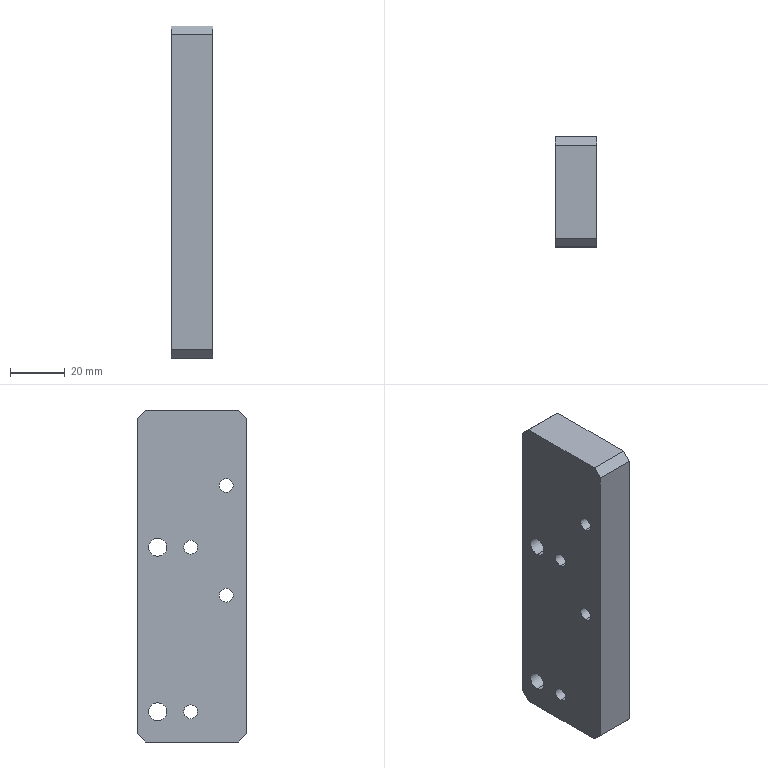Part | SolidWorks | features HoleWzd 4, Chamfer 1, Extrusion 1 | 1 solid | 44 faces | box 15 x 40 x 121 mm | volume 68938 mm3 | cylinder 20 | cone 12 | plane 12 | commonest cylinder face diameters 5 x8 4.2 x4 6.6 x4 11 x4
STEP:
#1=CARTESIAN_POINT('',(14.8,0.5,13.));
#2=VERTEX_POINT('',#1);
#3=CARTESIAN_POINT('',(14.8,0.5,8.));
#4=VERTEX_POINT('',#3);
#5=CARTESIAN_POINT('',(14.8,0.5,10.5));
#6=DIRECTION('',(1.,0.,0.));
#7=DIRECTION('',(0.,0.,-1.));
#8=AXIS2_PLACEMENT_3D('',#5,#6,#7);
#9=CIRCLE('',#8,2.5);
#10=EDGE_CURVE('',#2,#4,#9,.T.);
#11=ORIENTED_EDGE('',*,*,#10,.F.);
#12=CARTESIAN_POINT('',(15.,0.5,13.2));
#13=VERTEX_POINT('',#12);
#14=CARTESIAN_POINT('',(15.,0.5,13.2));
#15=DIRECTION('',(0.7071,0.,0.7071));
#16=VECTOR('',#15,1000.);
#17=LINE('',#14,#16);
#18=EDGE_CURVE('',#2,#13,#17,.T.);
#19=ORIENTED_EDGE('',*,*,#18,.T.);
#20=CARTESIAN_POINT('',(15.,0.5,7.8));
#21=VERTEX_POINT('',#20);
#22=CARTESIAN_POINT('',(15.,0.5,10.5));
#23=DIRECTION('',(1.,0.,0.));
#24=DIRECTION('',(0.,0.,-1.));
#25=AXIS2_PLACEMENT_3D('',#22,#23,#24);
#26=CIRCLE('',#25,2.7);
#27=EDGE_CURVE('',#13,#21,#26,.T.);
#28=ORIENTED_EDGE('',*,*,#27,.T.);
#29=CARTESIAN_POINT('',(15.,0.5,7.8));
#30=DIRECTION('',(0.7071,0.,-0.7071));
#31=VECTOR('',#30,1000.);
#32=LINE('',#29,#31);
#33=EDGE_CURVE('',#4,#21,#32,.T.);
#34=ORIENTED_EDGE('',*,*,#33,.F.);
#35=EDGE_LOOP('',(#11,#19,#28,#34));
#36=FACE_OUTER_BOUND('',#35,.T.);
#37=CARTESIAN_POINT('',(15.,0.5,10.5));
#38=DIRECTION('',(1.,0.,0.));
#39=DIRECTION('',(0.,0.,-1.));
#40=AXIS2_PLACEMENT_3D('',#37,#38,#39);
#41=CONICAL_SURFACE('',#40,2.7,0.7854);
#42=ADVANCED_FACE('',(#36),#41,.F.);
#43=CARTESIAN_POINT('',(0.,0.5,13.));
#44=VERTEX_POINT('',#43);
#45=CARTESIAN_POINT('',(0.,0.5,8.));
#46=VERTEX_POINT('',#45);
#47=CARTESIAN_POINT('',(0.,0.5,10.5));
#48=DIRECTION('',(1.,0.,0.));
#49=DIRECTION('',(0.,0.,-1.));
#50=AXIS2_PLACEMENT_3D('',#47,#48,#49);
#51=CIRCLE('',#50,2.5);
#52=EDGE_CURVE('',#44,#46,#51,.T.);
#53=ORIENTED_EDGE('',*,*,#52,.F.);
#54=CARTESIAN_POINT('',(15.,0.5,13.));
#55=DIRECTION('',(1.,0.,0.));
#56=VECTOR('',#55,1000.);
#57=LINE('',#54,#56);
#58=EDGE_CURVE('',#44,#2,#57,.T.);
#59=ORIENTED_EDGE('',*,*,#58,.T.);
#60=ORIENTED_EDGE('',*,*,#10,.T.);
#61=CARTESIAN_POINT('',(15.,0.5,8.));
#62=DIRECTION('',(1.,0.,0.));
#63=VECTOR('',#62,1000.);
#64=LINE('',#61,#63);
#65=EDGE_CURVE('',#46,#4,#64,.T.);
#66=ORIENTED_EDGE('',*,*,#65,.F.);
#67=EDGE_LOOP('',(#53,#59,#60,#66));
#68=FACE_OUTER_BOUND('',#67,.T.);
#69=CARTESIAN_POINT('',(15.,0.5,10.5));
#70=DIRECTION('',(1.,0.,0.));
#71=DIRECTION('',(0.,0.,-1.));
#72=AXIS2_PLACEMENT_3D('',#69,#70,#71);
#73=CYLINDRICAL_SURFACE('',#72,2.5);
#74=ADVANCED_FACE('',(#68),#73,.F.);
#75=CARTESIAN_POINT('',(14.8,0.5,-47.));
#76=VERTEX_POINT('',#75);
#77=CARTESIAN_POINT('',(14.8,0.5,-52.));
#78=VERTEX_POINT('',#77);
#79=CARTESIAN_POINT('',(14.8,0.5,-49.5));
#80=DIRECTION('',(1.,0.,0.));
#81=DIRECTION('',(0.,0.,-1.));
#82=AXIS2_PLACEMENT_3D('',#79,#80,#81);
#83=CIRCLE('',#82,2.5);
#84=EDGE_CURVE('',#76,#78,#83,.T.);
#85=ORIENTED_EDGE('',*,*,#84,.F.);
#86=CARTESIAN_POINT('',(15.,0.5,-46.8));
#87=VERTEX_POINT('',#86);
#88=CARTESIAN_POINT('',(15.,0.5,-46.8));
#89=DIRECTION('',(0.7071,0.,0.7071));
#90=VECTOR('',#89,1000.);
#91=LINE('',#88,#90);
#92=EDGE_CURVE('',#76,#87,#91,.T.);
#93=ORIENTED_EDGE('',*,*,#92,.T.);
#94=CARTESIAN_POINT('',(15.,0.5,-52.2));
#95=VERTEX_POINT('',#94);
#96=CARTESIAN_POINT('',(15.,0.5,-49.5));
#97=DIRECTION('',(1.,0.,0.));
#98=DIRECTION('',(0.,0.,-1.));
#99=AXIS2_PLACEMENT_3D('',#96,#97,#98);
#100=CIRCLE('',#99,2.7);
#101=EDGE_CURVE('',#87,#95,#100,.T.);
#102=ORIENTED_EDGE('',*,*,#101,.T.);
#103=CARTESIAN_POINT('',(15.,0.5,-52.2));
#104=DIRECTION('',(0.7071,0.,-0.7071));
#105=VECTOR('',#104,1000.);
#106=LINE('',#103,#105);
#107=EDGE_CURVE('',#78,#95,#106,.T.);
#108=ORIENTED_EDGE('',*,*,#107,.F.);
#109=EDGE_LOOP('',(#85,#93,#102,#108));
#110=FACE_OUTER_BOUND('',#109,.T.);
#111=CARTESIAN_POINT('',(15.,0.5,-49.5));
#112=DIRECTION('',(1.,0.,0.));
#113=DIRECTION('',(0.,0.,-1.));
#114=AXIS2_PLACEMENT_3D('',#111,#112,#113);
#115=CONICAL_SURFACE('',#114,2.7,0.7854);
#116=ADVANCED_FACE('',(#110),#115,.F.);
#117=CARTESIAN_POINT('',(0.,0.5,-47.));
#118=VERTEX_POINT('',#117);
#119=CARTESIAN_POINT('',(0.,0.5,-52.));
#120=VERTEX_POINT('',#119);
#121=CARTESIAN_POINT('',(0.,0.5,-49.5));
#122=DIRECTION('',(1.,0.,0.));
#123=DIRECTION('',(0.,0.,-1.));
#124=AXIS2_PLACEMENT_3D('',#121,#122,#123);
#125=CIRCLE('',#124,2.5);
#126=EDGE_CURVE('',#118,#120,#125,.T.);
#127=ORIENTED_EDGE('',*,*,#126,.F.);
#128=CARTESIAN_POINT('',(15.,0.5,-47.));
#129=DIRECTION('',(1.,0.,0.));
#130=VECTOR('',#129,1000.);
#131=LINE('',#128,#130);
#132=EDGE_CURVE('',#118,#76,#131,.T.);
#133=ORIENTED_EDGE('',*,*,#132,.T.);
#134=ORIENTED_EDGE('',*,*,#84,.T.);
#135=CARTESIAN_POINT('',(15.,0.5,-52.));
#136=DIRECTION('',(1.,0.,0.));
#137=VECTOR('',#136,1000.);
#138=LINE('',#135,#137);
#139=EDGE_CURVE('',#120,#78,#138,.T.);
#140=ORIENTED_EDGE('',*,*,#139,.F.);
#141=EDGE_LOOP('',(#127,#133,#134,#140));
#142=FACE_OUTER_BOUND('',#141,.T.);
#143=CARTESIAN_POINT('',(15.,0.5,-49.5));
#144=DIRECTION('',(1.,0.,0.));
#145=DIRECTION('',(0.,0.,-1.));
#146=AXIS2_PLACEMENT_3D('',#143,#144,#145);
#147=CYLINDRICAL_SURFACE('',#146,2.5);
#148=ADVANCED_FACE('',(#142),#147,.F.);
#149=CARTESIAN_POINT('',(8.2,12.5,16.));
#150=VERTEX_POINT('',#149);
#151=CARTESIAN_POINT('',(8.2,12.5,5.));
#152=VERTEX_POINT('',#151);
#153=CARTESIAN_POINT('',(8.2,12.5,10.5));
#154=DIRECTION('',(1.,0.,0.));
#155=DIRECTION('',(0.,0.,-1.));
#156=AXIS2_PLACEMENT_3D('',#153,#154,#155);
#157=CIRCLE('',#156,5.5);
#158=EDGE_CURVE('',#150,#152,#157,.T.);
#159=ORIENTED_EDGE('',*,*,#158,.F.);
#160=CARTESIAN_POINT('',(15.,12.5,16.));
#161=VERTEX_POINT('',#160);
#162=CARTESIAN_POINT('',(15.,12.5,16.));
#163=DIRECTION('',(1.,0.,0.));
#164=VECTOR('',#163,1000.);
#165=LINE('',#162,#164);
#166=EDGE_CURVE('',#150,#161,#165,.T.);
#167=ORIENTED_EDGE('',*,*,#166,.T.);
#168=CARTESIAN_POINT('',(15.,12.5,5.));
#169=VERTEX_POINT('',#168);
#170=CARTESIAN_POINT('',(15.,12.5,10.5));
#171=DIRECTION('',(1.,0.,0.));
#172=DIRECTION('',(0.,0.,-1.));
#173=AXIS2_PLACEMENT_3D('',#170,#171,#172);
#174=CIRCLE('',#173,5.5);
#175=EDGE_CURVE('',#161,#169,#174,.T.);
#176=ORIENTED_EDGE('',*,*,#175,.T.);
#177=CARTESIAN_POINT('',(15.,12.5,5.));
#178=DIRECTION('',(1.,0.,0.));
#179=VECTOR('',#178,1000.);
#180=LINE('',#177,#179);
#181=EDGE_CURVE('',#152,#169,#180,.T.);
#182=ORIENTED_EDGE('',*,*,#181,.F.);
#183=EDGE_LOOP('',(#159,#167,#176,#182));
#184=FACE_OUTER_BOUND('',#183,.T.);
#185=CARTESIAN_POINT('',(15.,12.5,10.5));
#186=DIRECTION('',(1.,0.,0.));
#187=DIRECTION('',(0.,0.,-1.));
#188=AXIS2_PLACEMENT_3D('',#185,#186,#187);
#189=CYLINDRICAL_SURFACE('',#188,5.5);
#190=ADVANCED_FACE('',(#184),#189,.F.);
#191=CARTESIAN_POINT('',(0.,12.5,13.8));
#192=VERTEX_POINT('',#191);
#193=CARTESIAN_POINT('',(0.,12.5,7.2));
#194=VERTEX_POINT('',#193);
#195=CARTESIAN_POINT('',(0.,12.5,10.5));
#196=DIRECTION('',(1.,0.,0.));
#197=DIRECTION('',(0.,0.,-1.));
#198=AXIS2_PLACEMENT_3D('',#195,#196,#197);
#199=CIRCLE('',#198,3.3);
#200=EDGE_CURVE('',#192,#194,#199,.T.);
#201=ORIENTED_EDGE('',*,*,#200,.F.);
#202=CARTESIAN_POINT('',(8.2,12.5,13.8));
#203=VERTEX_POINT('',#202);
#204=CARTESIAN_POINT('',(15.,12.5,13.8));
#205=DIRECTION('',(1.,0.,0.));
#206=VECTOR('',#205,1000.);
#207=LINE('',#204,#206);
#208=EDGE_CURVE('',#192,#203,#207,.T.);
#209=ORIENTED_EDGE('',*,*,#208,.T.);
#210=CARTESIAN_POINT('',(8.2,12.5,7.2));
#211=VERTEX_POINT('',#210);
#212=CARTESIAN_POINT('',(8.2,12.5,10.5));
#213=DIRECTION('',(1.,0.,0.));
#214=DIRECTION('',(0.,0.,-1.));
#215=AXIS2_PLACEMENT_3D('',#212,#213,#214);
#216=CIRCLE('',#215,3.3);
#217=EDGE_CURVE('',#203,#211,#216,.T.);
#218=ORIENTED_EDGE('',*,*,#217,.T.);
#219=CARTESIAN_POINT('',(15.,12.5,7.2));
#220=DIRECTION('',(1.,0.,0.));
#221=VECTOR('',#220,1000.);
#222=LINE('',#219,#221);
#223=EDGE_CURVE('',#194,#211,#222,.T.);
#224=ORIENTED_EDGE('',*,*,#223,.F.);
#225=EDGE_LOOP('',(#201,#209,#218,#224));
#226=FACE_OUTER_BOUND('',#225,.T.);
#227=CARTESIAN_POINT('',(15.,12.5,10.5));
#228=DIRECTION('',(1.,0.,0.));
#229=DIRECTION('',(0.,0.,-1.));
#230=AXIS2_PLACEMENT_3D('',#227,#228,#229);
#231=CYLINDRICAL_SURFACE('',#230,3.3);
#232=ADVANCED_FACE('',(#226),#231,.F.);
#233=CARTESIAN_POINT('',(8.2,12.5,-44.));
#234=VERTEX_POINT('',#233);
#235=CARTESIAN_POINT('',(8.2,12.5,-55.));
#236=VERTEX_POINT('',#235);
#237=CARTESIAN_POINT('',(8.2,12.5,-49.5));
#238=DIRECTION('',(1.,0.,0.));
#239=DIRECTION('',(0.,0.,-1.));
#240=AXIS2_PLACEMENT_3D('',#237,#238,#239);
#241=CIRCLE('',#240,5.5);
#242=EDGE_CURVE('',#234,#236,#241,.T.);
#243=ORIENTED_EDGE('',*,*,#242,.F.);
#244=CARTESIAN_POINT('',(15.,12.5,-44.));
#245=VERTEX_POINT('',#244);
#246=CARTESIAN_POINT('',(15.,12.5,-44.));
#247=DIRECTION('',(1.,0.,0.));
#248=VECTOR('',#247,1000.);
#249=LINE('',#246,#248);
#250=EDGE_CURVE('',#234,#245,#249,.T.);
#251=ORIENTED_EDGE('',*,*,#250,.T.);
#252=CARTESIAN_POINT('',(15.,12.5,-55.));
#253=VERTEX_POINT('',#252);
#254=CARTESIAN_POINT('',(15.,12.5,-49.5));
#255=DIRECTION('',(1.,0.,0.));
#256=DIRECTION('',(0.,0.,-1.));
#257=AXIS2_PLACEMENT_3D('',#254,#255,#256);
#258=CIRCLE('',#257,5.5);
#259=EDGE_CURVE('',#245,#253,#258,.T.);
#260=ORIENTED_EDGE('',*,*,#259,.T.);
#261=CARTESIAN_POINT('',(15.,12.5,-55.));
#262=DIRECTION('',(1.,0.,0.));
#263=VECTOR('',#262,1000.);
#264=LINE('',#261,#263);
#265=EDGE_CURVE('',#236,#253,#264,.T.);
#266=ORIENTED_EDGE('',*,*,#265,.F.);
#267=EDGE_LOOP('',(#243,#251,#260,#266));
#268=FACE_OUTER_BOUND('',#267,.T.);
#269=CARTESIAN_POINT('',(15.,12.5,-49.5));
#270=DIRECTION('',(1.,0.,0.));
#271=DIRECTION('',(0.,0.,-1.));
#272=AXIS2_PLACEMENT_3D('',#269,#270,#271);
#273=CYLINDRICAL_SURFACE('',#272,5.5);
#274=ADVANCED_FACE('',(#268),#273,.F.);
#275=CARTESIAN_POINT('',(0.,12.5,-46.2));
#276=VERTEX_POINT('',#275);
#277=CARTESIAN_POINT('',(0.,12.5,-52.8));
#278=VERTEX_POINT('',#277);
#279=CARTESIAN_POINT('',(0.,12.5,-49.5));
#280=DIRECTION('',(1.,0.,0.));
#281=DIRECTION('',(0.,0.,-1.));
#282=AXIS2_PLACEMENT_3D('',#279,#280,#281);
#283=CIRCLE('',#282,3.3);
#284=EDGE_CURVE('',#276,#278,#283,.T.);
#285=ORIENTED_EDGE('',*,*,#284,.F.);
#286=CARTESIAN_POINT('',(8.2,12.5,-46.2));
#287=VERTEX_POINT('',#286);
#288=CARTESIAN_POINT('',(15.,12.5,-46.2));
#289=DIRECTION('',(1.,0.,0.));
#290=VECTOR('',#289,1000.);
#291=LINE('',#288,#290);
#292=EDGE_CURVE('',#276,#287,#291,.T.);
#293=ORIENTED_EDGE('',*,*,#292,.T.);
#294=CARTESIAN_POINT('',(8.2,12.5,-52.8));
#295=VERTEX_POINT('',#294);
#296=CARTESIAN_POINT('',(8.2,12.5,-49.5));
#297=DIRECTION('',(1.,0.,0.));
#298=DIRECTION('',(0.,0.,-1.));
#299=AXIS2_PLACEMENT_3D('',#296,#297,#298);
#300=CIRCLE('',#299,3.3);
#301=EDGE_CURVE('',#287,#295,#300,.T.);
#302=ORIENTED_EDGE('',*,*,#301,.T.);
#303=CARTESIAN_POINT('',(15.,12.5,-52.8));
#304=DIRECTION('',(1.,0.,0.));
#305=VECTOR('',#304,1000.);
#306=LINE('',#303,#305);
#307=EDGE_CURVE('',#278,#295,#306,.T.);
#308=ORIENTED_EDGE('',*,*,#307,.F.);
#309=EDGE_LOOP('',(#285,#293,#302,#308));
#310=FACE_OUTER_BOUND('',#309,.T.);
#311=CARTESIAN_POINT('',(15.,12.5,-49.5));
#312=DIRECTION('',(1.,0.,0.));
#313=DIRECTION('',(0.,0.,-1.));
#314=AXIS2_PLACEMENT_3D('',#311,#312,#313);
#315=CYLINDRICAL_SURFACE('',#314,3.3);
#316=ADVANCED_FACE('',(#310),#315,.F.);
#317=CARTESIAN_POINT('',(14.475,-12.5,35.5));
#318=VERTEX_POINT('',#317);
#319=CARTESIAN_POINT('',(14.475,-12.5,30.5));
#320=VERTEX_POINT('',#319);
#321=CARTESIAN_POINT('',(14.475,-12.5,33.));
#322=DIRECTION('',(1.,0.,0.));
#323=DIRECTION('',(0.,0.,-1.));
#324=AXIS2_PLACEMENT_3D('',#321,#322,#323);
#325=CIRCLE('',#324,2.5);
#326=EDGE_CURVE('',#318,#320,#325,.T.);
#327=ORIENTED_EDGE('',*,*,#326,.F.);
#328=CARTESIAN_POINT('',(15.,-12.5,36.025));
#329=VERTEX_POINT('',#328);
#330=CARTESIAN_POINT('',(15.,-12.5,36.025));
#331=DIRECTION('',(0.7071,0.,0.7071));
#332=VECTOR('',#331,1000.);
#333=LINE('',#330,#332);
#334=EDGE_CURVE('',#318,#329,#333,.T.);
#335=ORIENTED_EDGE('',*,*,#334,.T.);
#336=CARTESIAN_POINT('',(15.,-12.5,29.975));
#337=VERTEX_POINT('',#336);
#338=CARTESIAN_POINT('',(15.,-12.5,33.));
#339=DIRECTION('',(1.,0.,0.));
#340=DIRECTION('',(0.,0.,-1.));
#341=AXIS2_PLACEMENT_3D('',#338,#339,#340);
#342=CIRCLE('',#341,3.025);
#343=EDGE_CURVE('',#329,#337,#342,.T.);
#344=ORIENTED_EDGE('',*,*,#343,.T.);
#345=CARTESIAN_POINT('',(15.,-12.5,29.975));
#346=DIRECTION('',(0.7071,0.,-0.7071));
#347=VECTOR('',#346,1000.);
#348=LINE('',#345,#347);
#349=EDGE_CURVE('',#320,#337,#348,.T.);
#350=ORIENTED_EDGE('',*,*,#349,.F.);
#351=EDGE_LOOP('',(#327,#335,#344,#350));
#352=FACE_OUTER_BOUND('',#351,.T.);
#353=CARTESIAN_POINT('',(15.,-12.5,33.));
#354=DIRECTION('',(1.,0.,0.));
#355=DIRECTION('',(0.,0.,-1.));
#356=AXIS2_PLACEMENT_3D('',#353,#354,#355);
#357=CONICAL_SURFACE('',#356,3.025,0.7854);
#358=ADVANCED_FACE('',(#352),#357,.F.);
#359=CARTESIAN_POINT('',(0.,-12.5,35.5));
#360=VERTEX_POINT('',#359);
#361=CARTESIAN_POINT('',(0.,-12.5,30.5));
#362=VERTEX_POINT('',#361);
#363=CARTESIAN_POINT('',(0.,-12.5,33.));
#364=DIRECTION('',(1.,0.,0.));
#365=DIRECTION('',(0.,0.,-1.));
#366=AXIS2_PLACEMENT_3D('',#363,#364,#365);
#367=CIRCLE('',#366,2.5);
#368=EDGE_CURVE('',#360,#362,#367,.T.);
#369=ORIENTED_EDGE('',*,*,#368,.F.);
#370=CARTESIAN_POINT('',(15.,-12.5,35.5));
#371=DIRECTION('',(1.,0.,0.));
#372=VECTOR('',#371,1000.);
#373=LINE('',#370,#372);
#374=EDGE_CURVE('',#360,#318,#373,.T.);
#375=ORIENTED_EDGE('',*,*,#374,.T.);
#376=ORIENTED_EDGE('',*,*,#326,.T.);
#377=CARTESIAN_POINT('',(15.,-12.5,30.5));
#378=DIRECTION('',(1.,0.,0.));
#379=VECTOR('',#378,1000.);
#380=LINE('',#377,#379);
#381=EDGE_CURVE('',#362,#320,#380,.T.);
#382=ORIENTED_EDGE('',*,*,#381,.F.);
#383=EDGE_LOOP('',(#369,#375,#376,#382));
#384=FACE_OUTER_BOUND('',#383,.T.);
#385=CARTESIAN_POINT('',(15.,-12.5,33.));
#386=DIRECTION('',(1.,0.,0.));
#387=DIRECTION('',(0.,0.,-1.));
#388=AXIS2_PLACEMENT_3D('',#385,#386,#387);
#389=CYLINDRICAL_SURFACE('',#388,2.5);
#390=ADVANCED_FACE('',(#384),#389,.F.);
#391=CARTESIAN_POINT('',(14.475,-12.5,-4.5));
#392=VERTEX_POINT('',#391);
#393=CARTESIAN_POINT('',(14.475,-12.5,-9.5));
#394=VERTEX_POINT('',#393);
#395=CARTESIAN_POINT('',(14.475,-12.5,-7.));
#396=DIRECTION('',(1.,0.,0.));
#397=DIRECTION('',(0.,0.,-1.));
#398=AXIS2_PLACEMENT_3D('',#395,#396,#397);
#399=CIRCLE('',#398,2.5);
#400=EDGE_CURVE('',#392,#394,#399,.T.);
#401=ORIENTED_EDGE('',*,*,#400,.F.);
#402=CARTESIAN_POINT('',(15.,-12.5,-3.975));
#403=VERTEX_POINT('',#402);
#404=CARTESIAN_POINT('',(15.,-12.5,-3.975));
#405=DIRECTION('',(0.7071,0.,0.7071));
#406=VECTOR('',#405,1000.);
#407=LINE('',#404,#406);
#408=EDGE_CURVE('',#392,#403,#407,.T.);
#409=ORIENTED_EDGE('',*,*,#408,.T.);
#410=CARTESIAN_POINT('',(15.,-12.5,-10.025));
#411=VERTEX_POINT('',#410);
#412=CARTESIAN_POINT('',(15.,-12.5,-7.));
#413=DIRECTION('',(1.,0.,0.));
#414=DIRECTION('',(0.,0.,-1.));
#415=AXIS2_PLACEMENT_3D('',#412,#413,#414);
#416=CIRCLE('',#415,3.025);
#417=EDGE_CURVE('',#403,#411,#416,.T.);
#418=ORIENTED_EDGE('',*,*,#417,.T.);
#419=CARTESIAN_POINT('',(15.,-12.5,-10.025));
#420=DIRECTION('',(0.7071,0.,-0.7071));
#421=VECTOR('',#420,1000.);
#422=LINE('',#419,#421);
#423=EDGE_CURVE('',#394,#411,#422,.T.);
#424=ORIENTED_EDGE('',*,*,#423,.F.);
#425=EDGE_LOOP('',(#401,#409,#418,#424));
#426=FACE_OUTER_BOUND('',#425,.T.);
#427=CARTESIAN_POINT('',(15.,-12.5,-7.));
#428=DIRECTION('',(1.,0.,0.));
#429=DIRECTION('',(0.,0.,-1.));
#430=AXIS2_PLACEMENT_3D('',#427,#428,#429);
#431=CONICAL_SURFACE('',#430,3.025,0.7854);
#432=ADVANCED_FACE('',(#426),#431,.F.);
#433=CARTESIAN_POINT('',(0.,-12.5,-4.5));
#434=VERTEX_POINT('',#433);
#435=CARTESIAN_POINT('',(0.,-12.5,-9.5));
#436=VERTEX_POINT('',#435);
#437=CARTESIAN_POINT('',(0.,-12.5,-7.));
#438=DIRECTION('',(1.,0.,0.));
#439=DIRECTION('',(0.,0.,-1.));
#440=AXIS2_PLACEMENT_3D('',#437,#438,#439);
#441=CIRCLE('',#440,2.5);
#442=EDGE_CURVE('',#434,#436,#441,.T.);
#443=ORIENTED_EDGE('',*,*,#442,.F.);
#444=CARTESIAN_POINT('',(15.,-12.5,-4.5));
#445=DIRECTION('',(1.,0.,0.));
#446=VECTOR('',#445,1000.);
#447=LINE('',#444,#446);
#448=EDGE_CURVE('',#434,#392,#447,.T.);
#449=ORIENTED_EDGE('',*,*,#448,.T.);
#450=ORIENTED_EDGE('',*,*,#400,.T.);
#451=CARTESIAN_POINT('',(15.,-12.5,-9.5));
#452=DIRECTION('',(1.,0.,0.));
#453=VECTOR('',#452,1000.);
#454=LINE('',#451,#453);
#455=EDGE_CURVE('',#436,#394,#454,.T.);
#456=ORIENTED_EDGE('',*,*,#455,.F.);
#457=EDGE_LOOP('',(#443,#449,#450,#456));
#458=FACE_OUTER_BOUND('',#457,.T.);
#459=CARTESIAN_POINT('',(15.,-12.5,-7.));
#460=DIRECTION('',(1.,0.,0.));
#461=DIRECTION('',(0.,0.,-1.));
#462=AXIS2_PLACEMENT_3D('',#459,#460,#461);
#463=CYLINDRICAL_SURFACE('',#462,2.5);
#464=ADVANCED_FACE('',(#458),#463,.F.);
#465=CARTESIAN_POINT('',(2.6,13.,55.1));
#466=VERTEX_POINT('',#465);
#467=CARTESIAN_POINT('',(2.6,13.,50.9));
#468=VERTEX_POINT('',#467);
#469=CARTESIAN_POINT('',(2.6,13.,53.));
#470=DIRECTION('',(1.,0.,0.));
#471=DIRECTION('',(0.,0.,-1.));
#472=AXIS2_PLACEMENT_3D('',#469,#470,#471);
#473=CIRCLE('',#472,2.1);
#474=EDGE_CURVE('',#466,#468,#473,.T.);
#475=ORIENTED_EDGE('',*,*,#474,.F.);
#476=CARTESIAN_POINT('',(15.,13.,55.1));
#477=VERTEX_POINT('',#476);
#478=CARTESIAN_POINT('',(15.,13.,55.1));
#479=DIRECTION('',(1.,0.,0.));
#480=VECTOR('',#479,1000.);
#481=LINE('',#478,#480);
#482=EDGE_CURVE('',#466,#477,#481,.T.);
#483=ORIENTED_EDGE('',*,*,#482,.T.);
#484=CARTESIAN_POINT('',(15.,13.,50.9));
#485=VERTEX_POINT('',#484);
#486=CARTESIAN_POINT('',(15.,13.,53.));
#487=DIRECTION('',(1.,0.,0.));
#488=DIRECTION('',(0.,0.,-1.));
#489=AXIS2_PLACEMENT_3D('',#486,#487,#488);
#490=CIRCLE('',#489,2.1);
#491=EDGE_CURVE('',#477,#485,#490,.T.);
#492=ORIENTED_EDGE('',*,*,#491,.T.);
#493=CARTESIAN_POINT('',(15.,13.,50.9));
#494=DIRECTION('',(1.,0.,0.));
#495=VECTOR('',#494,1000.);
#496=LINE('',#493,#495);
#497=EDGE_CURVE('',#468,#485,#496,.T.);
#498=ORIENTED_EDGE('',*,*,#497,.F.);
#499=EDGE_LOOP('',(#475,#483,#492,#498));
#500=FACE_OUTER_BOUND('',#499,.T.);
#501=CARTESIAN_POINT('',(15.,13.,53.));
#502=DIRECTION('',(1.,0.,0.));
#503=DIRECTION('',(0.,0.,-1.));
#504=AXIS2_PLACEMENT_3D('',#501,#502,#503);
#505=CYLINDRICAL_SURFACE('',#504,2.1);
#506=ADVANCED_FACE('',(#500),#505,.F.);
#507=CARTESIAN_POINT('',(1.338,13.,53.));
#508=VERTEX_POINT('',#507);
#509=CARTESIAN_POINT('',(2.6,13.,50.9));
#510=DIRECTION('',(0.515,0.,-0.8572));
#511=VECTOR('',#510,1000.);
#512=LINE('',#509,#511);
#513=EDGE_CURVE('',#508,#468,#512,.T.);
#514=ORIENTED_EDGE('',*,*,#513,.F.);
#515=CARTESIAN_POINT('',(2.6,13.,55.1));
#516=DIRECTION('',(0.515,0.,0.8572));
#517=VECTOR('',#516,1000.);
#518=LINE('',#515,#517);
#519=EDGE_CURVE('',#508,#466,#518,.T.);
#520=ORIENTED_EDGE('',*,*,#519,.T.);
#521=ORIENTED_EDGE('',*,*,#474,.T.);
#522=EDGE_LOOP('',(#514,#520,#521));
#523=FACE_OUTER_BOUND('',#522,.T.);
#524=CARTESIAN_POINT('',(2.6,13.,53.));
#525=DIRECTION('',(1.,0.,0.));
#526=DIRECTION('',(0.,0.,-1.));
#527=AXIS2_PLACEMENT_3D('',#524,#525,#526);
#528=CONICAL_SURFACE('',#527,2.1,1.03);
#529=ADVANCED_FACE('',(#523),#528,.F.);
#530=CARTESIAN_POINT('',(2.6,13.,-24.9));
#531=VERTEX_POINT('',#530);
#532=CARTESIAN_POINT('',(2.6,13.,-29.1));
#533=VERTEX_POINT('',#532);
#534=CARTESIAN_POINT('',(2.6,13.,-27.));
#535=DIRECTION('',(1.,0.,0.));
#536=DIRECTION('',(0.,0.,-1.));
#537=AXIS2_PLACEMENT_3D('',#534,#535,#536);
#538=CIRCLE('',#537,2.1);
#539=EDGE_CURVE('',#531,#533,#538,.T.);
#540=ORIENTED_EDGE('',*,*,#539,.F.);
#541=CARTESIAN_POINT('',(15.,13.,-24.9));
#542=VERTEX_POINT('',#541);
#543=CARTESIAN_POINT('',(15.,13.,-24.9));
#544=DIRECTION('',(1.,0.,0.));
#545=VECTOR('',#544,1000.);
#546=LINE('',#543,#545);
#547=EDGE_CURVE('',#531,#542,#546,.T.);
#548=ORIENTED_EDGE('',*,*,#547,.T.);
#549=CARTESIAN_POINT('',(15.,13.,-29.1));
#550=VERTEX_POINT('',#549);
#551=CARTESIAN_POINT('',(15.,13.,-27.));
#552=DIRECTION('',(1.,0.,0.));
#553=DIRECTION('',(0.,0.,-1.));
#554=AXIS2_PLACEMENT_3D('',#551,#552,#553);
#555=CIRCLE('',#554,2.1);
#556=EDGE_CURVE('',#542,#550,#555,.T.);
#557=ORIENTED_EDGE('',*,*,#556,.T.);
#558=CARTESIAN_POINT('',(15.,13.,-29.1));
#559=DIRECTION('',(1.,0.,0.));
#560=VECTOR('',#559,1000.);
#561=LINE('',#558,#560);
#562=EDGE_CURVE('',#533,#550,#561,.T.);
#563=ORIENTED_EDGE('',*,*,#562,.F.);
#564=EDGE_LOOP('',(#540,#548,#557,#563));
#565=FACE_OUTER_BOUND('',#564,.T.);
#566=CARTESIAN_POINT('',(15.,13.,-27.));
#567=DIRECTION('',(1.,0.,0.));
#568=DIRECTION('',(0.,0.,-1.));
#569=AXIS2_PLACEMENT_3D('',#566,#567,#568);
#570=CYLINDRICAL_SURFACE('',#569,2.1);
#571=ADVANCED_FACE('',(#565),#570,.F.);
#572=CARTESIAN_POINT('',(1.338,13.,-27.));
#573=VERTEX_POINT('',#572);
#574=CARTESIAN_POINT('',(2.6,13.,-29.1));
#575=DIRECTION('',(0.515,0.,-0.8572));
#576=VECTOR('',#575,1000.);
#577=LINE('',#574,#576);
#578=EDGE_CURVE('',#573,#533,#577,.T.);
#579=ORIENTED_EDGE('',*,*,#578,.F.);
#580=CARTESIAN_POINT('',(2.6,13.,-24.9));
#581=DIRECTION('',(0.515,0.,0.8572));
#582=VECTOR('',#581,1000.);
#583=LINE('',#580,#582);
#584=EDGE_CURVE('',#573,#531,#583,.T.);
#585=ORIENTED_EDGE('',*,*,#584,.T.);
#586=ORIENTED_EDGE('',*,*,#539,.T.);
#587=EDGE_LOOP('',(#579,#585,#586));
#588=FACE_OUTER_BOUND('',#587,.T.);
#589=CARTESIAN_POINT('',(2.6,13.,-27.));
#590=DIRECTION('',(1.,0.,0.));
#591=DIRECTION('',(0.,0.,-1.));
#592=AXIS2_PLACEMENT_3D('',#589,#590,#591);
#593=CONICAL_SURFACE('',#592,2.1,1.03);
#594=ADVANCED_FACE('',(#588),#593,.F.);
#595=CARTESIAN_POINT('',(0.,-17.,-60.5));
#596=VERTEX_POINT('',#595);
#597=CARTESIAN_POINT('',(0.,17.,-60.5));
#598=VERTEX_POINT('',#597);
#599=CARTESIAN_POINT('',(0.,-20.,-60.5));
#600=DIRECTION('',(0.,1.,0.));
#601=VECTOR('',#600,1000.);
#602=LINE('',#599,#601);
#603=EDGE_CURVE('',#596,#598,#602,.T.);
#604=ORIENTED_EDGE('',*,*,#603,.T.);
#605=CARTESIAN_POINT('',(15.,17.,-60.5));
#606=VERTEX_POINT('',#605);
#607=CARTESIAN_POINT('',(15.,17.,-60.5));
#608=DIRECTION('',(1.,0.,0.));
#609=VECTOR('',#608,1000.);
#610=LINE('',#607,#609);
#611=EDGE_CURVE('',#598,#606,#610,.T.);
#612=ORIENTED_EDGE('',*,*,#611,.T.);
#613=CARTESIAN_POINT('',(15.,-17.,-60.5));
#614=VERTEX_POINT('',#613);
#615=CARTESIAN_POINT('',(15.,-20.,-60.5));
#616=DIRECTION('',(0.,1.,0.));
#617=VECTOR('',#616,1000.);
#618=LINE('',#615,#617);
#619=EDGE_CURVE('',#614,#606,#618,.T.);
#620=ORIENTED_EDGE('',*,*,#619,.F.);
#621=CARTESIAN_POINT('',(15.,-17.,-60.5));
#622=DIRECTION('',(-1.,0.,0.));
#623=VECTOR('',#622,1000.);
#624=LINE('',#621,#623);
#625=EDGE_CURVE('',#614,#596,#624,.T.);
#626=ORIENTED_EDGE('',*,*,#625,.T.);
#627=EDGE_LOOP('',(#604,#612,#620,#626));
#628=FACE_OUTER_BOUND('',#627,.T.);
#629=CARTESIAN_POINT('',(15.,-20.,-60.5));
#630=DIRECTION('',(0.,0.,1.));
#631=DIRECTION('',(1.,0.,0.));
#632=AXIS2_PLACEMENT_3D('',#629,#630,#631);
#633=PLANE('',#632);
#634=ADVANCED_FACE('',(#628),#633,.F.);
#635=CARTESIAN_POINT('',(15.,20.,-57.5));
#636=VERTEX_POINT('',#635);
#637=CARTESIAN_POINT('',(15.,20.,57.5));
#638=VERTEX_POINT('',#637);
#639=CARTESIAN_POINT('',(15.,20.,60.5));
#640=DIRECTION('',(0.,0.,1.));
#641=VECTOR('',#640,1000.);
#642=LINE('',#639,#641);
#643=EDGE_CURVE('',#636,#638,#642,.T.);
#644=ORIENTED_EDGE('',*,*,#643,.F.);
#645=CARTESIAN_POINT('',(0.,20.,-57.5));
#646=VERTEX_POINT('',#645);
#647=CARTESIAN_POINT('',(15.,20.,-57.5));
#648=DIRECTION('',(-1.,0.,0.));
#649=VECTOR('',#648,1000.);
#650=LINE('',#647,#649);
#651=EDGE_CURVE('',#636,#646,#650,.T.);
#652=ORIENTED_EDGE('',*,*,#651,.T.);
#653=CARTESIAN_POINT('',(0.,20.,57.5));
#654=VERTEX_POINT('',#653);
#655=CARTESIAN_POINT('',(0.,20.,60.5));
#656=DIRECTION('',(0.,0.,1.));
#657=VECTOR('',#656,1000.);
#658=LINE('',#655,#657);
#659=EDGE_CURVE('',#646,#654,#658,.T.);
#660=ORIENTED_EDGE('',*,*,#659,.T.);
#661=CARTESIAN_POINT('',(15.,20.,57.5));
#662=DIRECTION('',(1.,0.,0.));
#663=VECTOR('',#662,1000.);
#664=LINE('',#661,#663);
#665=EDGE_CURVE('',#654,#638,#664,.T.);
#666=ORIENTED_EDGE('',*,*,#665,.T.);
#667=EDGE_LOOP('',(#644,#652,#660,#666));
#668=FACE_OUTER_BOUND('',#667,.T.);
#669=CARTESIAN_POINT('',(15.,20.,60.5));
#670=DIRECTION('',(0.,-1.,0.));
#671=DIRECTION('',(0.,0.,-1.));
#672=AXIS2_PLACEMENT_3D('',#669,#670,#671);
#673=PLANE('',#672);
#674=ADVANCED_FACE('',(#668),#673,.F.);
#675=CARTESIAN_POINT('',(15.,17.,60.5));
#676=VERTEX_POINT('',#675);
#677=CARTESIAN_POINT('',(15.,-17.,60.5));
#678=VERTEX_POINT('',#677);
#679=CARTESIAN_POINT('',(15.,-20.,60.5));
#680=DIRECTION('',(0.,-1.,0.));
#681=VECTOR('',#680,1000.);
#682=LINE('',#679,#681);
#683=EDGE_CURVE('',#676,#678,#682,.T.);
#684=ORIENTED_EDGE('',*,*,#683,.F.);
#685=CARTESIAN_POINT('',(0.,17.,60.5));
#686=VERTEX_POINT('',#685);
#687=CARTESIAN_POINT('',(15.,17.,60.5));
#688=DIRECTION('',(-1.,0.,0.));
#689=VECTOR('',#688,1000.);
#690=LINE('',#687,#689);
#691=EDGE_CURVE('',#676,#686,#690,.T.);
#692=ORIENTED_EDGE('',*,*,#691,.T.);
#693=CARTESIAN_POINT('',(0.,-17.,60.5));
#694=VERTEX_POINT('',#693);
#695=CARTESIAN_POINT('',(0.,-20.,60.5));
#696=DIRECTION('',(0.,-1.,0.));
#697=VECTOR('',#696,1000.);
#698=LINE('',#695,#697);
#699=EDGE_CURVE('',#686,#694,#698,.T.);
#700=ORIENTED_EDGE('',*,*,#699,.T.);
#701=CARTESIAN_POINT('',(15.,-17.,60.5));
#702=DIRECTION('',(1.,0.,0.));
#703=VECTOR('',#702,1000.);
#704=LINE('',#701,#703);
#705=EDGE_CURVE('',#694,#678,#704,.T.);
#706=ORIENTED_EDGE('',*,*,#705,.T.);
#707=EDGE_LOOP('',(#684,#692,#700,#706));
#708=FACE_OUTER_BOUND('',#707,.T.);
#709=CARTESIAN_POINT('',(15.,-20.,60.5));
#710=DIRECTION('',(0.,0.,-1.));
#711=DIRECTION('',(-1.,0.,0.));
#712=AXIS2_PLACEMENT_3D('',#709,#710,#711);
#713=PLANE('',#712);
#714=ADVANCED_FACE('',(#708),#713,.F.);
#715=CARTESIAN_POINT('',(0.,-20.,57.5));
#716=VERTEX_POINT('',#715);
#717=CARTESIAN_POINT('',(0.,-20.,-57.5));
#718=VERTEX_POINT('',#717);
#719=CARTESIAN_POINT('',(0.,-20.,60.5));
#720=DIRECTION('',(0.,0.,-1.));
#721=VECTOR('',#720,1000.);
#722=LINE('',#719,#721);
#723=EDGE_CURVE('',#716,#718,#722,.T.);
#724=ORIENTED_EDGE('',*,*,#723,.T.);
#725=CARTESIAN_POINT('',(15.,-20.,-57.5));
#726=VERTEX_POINT('',#725);
#727=CARTESIAN_POINT('',(15.,-20.,-57.5));
#728=DIRECTION('',(1.,0.,0.));
#729=VECTOR('',#728,1000.);
#730=LINE('',#727,#729);
#731=EDGE_CURVE('',#718,#726,#730,.T.);
#732=ORIENTED_EDGE('',*,*,#731,.T.);
#733=CARTESIAN_POINT('',(15.,-20.,57.5));
#734=VERTEX_POINT('',#733);
#735=CARTESIAN_POINT('',(15.,-20.,60.5));
#736=DIRECTION('',(0.,0.,-1.));
#737=VECTOR('',#736,1000.);
#738=LINE('',#735,#737);
#739=EDGE_CURVE('',#734,#726,#738,.T.);
#740=ORIENTED_EDGE('',*,*,#739,.F.);
#741=CARTESIAN_POINT('',(15.,-20.,57.5));
#742=DIRECTION('',(-1.,0.,0.));
#743=VECTOR('',#742,1000.);
#744=LINE('',#741,#743);
#745=EDGE_CURVE('',#734,#716,#744,.T.);
#746=ORIENTED_EDGE('',*,*,#745,.T.);
#747=EDGE_LOOP('',(#724,#732,#740,#746));
#748=FACE_OUTER_BOUND('',#747,.T.);
#749=CARTESIAN_POINT('',(15.,-20.,60.5));
#750=DIRECTION('',(0.,1.,0.));
#751=DIRECTION('',(0.,0.,1.));
#752=AXIS2_PLACEMENT_3D('',#749,#750,#751);
#753=PLANE('',#752);
#754=ADVANCED_FACE('',(#748),#753,.F.);
#755=CARTESIAN_POINT('',(15.,0.5,10.5));
#756=DIRECTION('',(1.,0.,0.));
#757=DIRECTION('',(0.,0.,-1.));
#758=AXIS2_PLACEMENT_3D('',#755,#756,#757);
#759=CIRCLE('',#758,2.7);
#760=EDGE_CURVE('',#21,#13,#759,.T.);
#761=ORIENTED_EDGE('',*,*,#760,.F.);
#762=ORIENTED_EDGE('',*,*,#27,.F.);
#763=EDGE_LOOP('',(#761,#762));
#764=FACE_BOUND('',#763,.T.);
#765=CARTESIAN_POINT('',(15.,0.5,-49.5));
#766=DIRECTION('',(1.,0.,0.));
#767=DIRECTION('',(0.,0.,-1.));
#768=AXIS2_PLACEMENT_3D('',#765,#766,#767);
#769=CIRCLE('',#768,2.7);
#770=EDGE_CURVE('',#95,#87,#769,.T.);
#771=ORIENTED_EDGE('',*,*,#770,.F.);
#772=ORIENTED_EDGE('',*,*,#101,.F.);
#773=EDGE_LOOP('',(#771,#772));
#774=FACE_BOUND('',#773,.T.);
#775=CARTESIAN_POINT('',(15.,12.5,10.5));
#776=DIRECTION('',(1.,0.,0.));
#777=DIRECTION('',(0.,0.,-1.));
#778=AXIS2_PLACEMENT_3D('',#775,#776,#777);
#779=CIRCLE('',#778,5.5);
#780=EDGE_CURVE('',#169,#161,#779,.T.);
#781=ORIENTED_EDGE('',*,*,#780,.F.);
#782=ORIENTED_EDGE('',*,*,#175,.F.);
#783=EDGE_LOOP('',(#781,#782));
#784=FACE_BOUND('',#783,.T.);
#785=CARTESIAN_POINT('',(15.,12.5,-49.5));
#786=DIRECTION('',(1.,0.,0.));
#787=DIRECTION('',(0.,0.,-1.));
#788=AXIS2_PLACEMENT_3D('',#785,#786,#787);
#789=CIRCLE('',#788,5.5);
#790=EDGE_CURVE('',#253,#245,#789,.T.);
#791=ORIENTED_EDGE('',*,*,#790,.F.);
#792=ORIENTED_EDGE('',*,*,#259,.F.);
#793=EDGE_LOOP('',(#791,#792));
#794=FACE_BOUND('',#793,.T.);
#795=CARTESIAN_POINT('',(15.,-12.5,33.));
#796=DIRECTION('',(1.,0.,0.));
#797=DIRECTION('',(0.,0.,-1.));
#798=AXIS2_PLACEMENT_3D('',#795,#796,#797);
#799=CIRCLE('',#798,3.025);
#800=EDGE_CURVE('',#337,#329,#799,.T.);
#801=ORIENTED_EDGE('',*,*,#800,.F.);
#802=ORIENTED_EDGE('',*,*,#343,.F.);
#803=EDGE_LOOP('',(#801,#802));
#804=FACE_BOUND('',#803,.T.);
#805=CARTESIAN_POINT('',(15.,-12.5,-7.));
#806=DIRECTION('',(1.,0.,0.));
#807=DIRECTION('',(0.,0.,-1.));
#808=AXIS2_PLACEMENT_3D('',#805,#806,#807);
#809=CIRCLE('',#808,3.025);
#810=EDGE_CURVE('',#411,#403,#809,.T.);
#811=ORIENTED_EDGE('',*,*,#810,.F.);
#812=ORIENTED_EDGE('',*,*,#417,.F.);
#813=EDGE_LOOP('',(#811,#812));
#814=FACE_BOUND('',#813,.T.);
#815=CARTESIAN_POINT('',(15.,13.,53.));
#816=DIRECTION('',(1.,0.,0.));
#817=DIRECTION('',(0.,0.,-1.));
#818=AXIS2_PLACEMENT_3D('',#815,#816,#817);
#819=CIRCLE('',#818,2.1);
#820=EDGE_CURVE('',#485,#477,#819,.T.);
#821=ORIENTED_EDGE('',*,*,#820,.F.);
#822=ORIENTED_EDGE('',*,*,#491,.F.);
#823=EDGE_LOOP('',(#821,#822));
#824=FACE_BOUND('',#823,.T.);
#825=CARTESIAN_POINT('',(15.,13.,-27.));
#826=DIRECTION('',(1.,0.,0.));
#827=DIRECTION('',(0.,0.,-1.));
#828=AXIS2_PLACEMENT_3D('',#825,#826,#827);
#829=CIRCLE('',#828,2.1);
#830=EDGE_CURVE('',#550,#542,#829,.T.);
#831=ORIENTED_EDGE('',*,*,#830,.F.);
#832=ORIENTED_EDGE('',*,*,#556,.F.);
#833=EDGE_LOOP('',(#831,#832));
#834=FACE_BOUND('',#833,.T.);
#835=ORIENTED_EDGE('',*,*,#619,.T.);
#836=CARTESIAN_POINT('',(15.,20.,-57.5));
#837=DIRECTION('',(0.,0.7071,0.7071));
#838=VECTOR('',#837,1000.);
#839=LINE('',#836,#838);
#840=EDGE_CURVE('',#606,#636,#839,.T.);
#841=ORIENTED_EDGE('',*,*,#840,.T.);
#842=ORIENTED_EDGE('',*,*,#643,.T.);
#843=CARTESIAN_POINT('',(15.,17.,60.5));
#844=DIRECTION('',(0.,-0.7071,0.7071));
#845=VECTOR('',#844,1000.);
#846=LINE('',#843,#845);
#847=EDGE_CURVE('',#638,#676,#846,.T.);
#848=ORIENTED_EDGE('',*,*,#847,.T.);
#849=ORIENTED_EDGE('',*,*,#683,.T.);
#850=CARTESIAN_POINT('',(15.,-20.,57.5));
#851=DIRECTION('',(0.,-0.7071,-0.7071));
#852=VECTOR('',#851,1000.);
#853=LINE('',#850,#852);
#854=EDGE_CURVE('',#678,#734,#853,.T.);
#855=ORIENTED_EDGE('',*,*,#854,.T.);
#856=ORIENTED_EDGE('',*,*,#739,.T.);
#857=CARTESIAN_POINT('',(15.,-17.,-60.5));
#858=DIRECTION('',(0.,0.7071,-0.7071));
#859=VECTOR('',#858,1000.);
#860=LINE('',#857,#859);
#861=EDGE_CURVE('',#726,#614,#860,.T.);
#862=ORIENTED_EDGE('',*,*,#861,.T.);
#863=EDGE_LOOP('',(#835,#841,#842,#848,#849,#855,#856,#862));
#864=FACE_OUTER_BOUND('',#863,.T.);
#865=CARTESIAN_POINT('',(15.,0.,0.));
#866=DIRECTION('',(-1.,0.,0.));
#867=DIRECTION('',(0.,0.,1.));
#868=AXIS2_PLACEMENT_3D('',#865,#866,#867);
#869=PLANE('',#868);
#870=ADVANCED_FACE('',(#764,#774,#784,#794,#804,#814,#824,#834,#864),#869,.F.);
#871=CARTESIAN_POINT('',(0.,0.5,10.5));
#872=DIRECTION('',(1.,0.,0.));
#873=DIRECTION('',(0.,0.,-1.));
#874=AXIS2_PLACEMENT_3D('',#871,#872,#873);
#875=CIRCLE('',#874,2.5);
#876=EDGE_CURVE('',#46,#44,#875,.T.);
#877=ORIENTED_EDGE('',*,*,#876,.T.);
#878=ORIENTED_EDGE('',*,*,#52,.T.);
#879=EDGE_LOOP('',(#877,#878));
#880=FACE_BOUND('',#879,.T.);
#881=CARTESIAN_POINT('',(0.,0.5,-49.5));
#882=DIRECTION('',(1.,0.,0.));
#883=DIRECTION('',(0.,0.,-1.));
#884=AXIS2_PLACEMENT_3D('',#881,#882,#883);
#885=CIRCLE('',#884,2.5);
#886=EDGE_CURVE('',#120,#118,#885,.T.);
#887=ORIENTED_EDGE('',*,*,#886,.T.);
#888=ORIENTED_EDGE('',*,*,#126,.T.);
#889=EDGE_LOOP('',(#887,#888));
#890=FACE_BOUND('',#889,.T.);
#891=CARTESIAN_POINT('',(0.,12.5,10.5));
#892=DIRECTION('',(1.,0.,0.));
#893=DIRECTION('',(0.,0.,-1.));
#894=AXIS2_PLACEMENT_3D('',#891,#892,#893);
#895=CIRCLE('',#894,3.3);
#896=EDGE_CURVE('',#194,#192,#895,.T.);
#897=ORIENTED_EDGE('',*,*,#896,.T.);
#898=ORIENTED_EDGE('',*,*,#200,.T.);
#899=EDGE_LOOP('',(#897,#898));
#900=FACE_BOUND('',#899,.T.);
#901=CARTESIAN_POINT('',(0.,12.5,-49.5));
#902=DIRECTION('',(1.,0.,0.));
#903=DIRECTION('',(0.,0.,-1.));
#904=AXIS2_PLACEMENT_3D('',#901,#902,#903);
#905=CIRCLE('',#904,3.3);
#906=EDGE_CURVE('',#278,#276,#905,.T.);
#907=ORIENTED_EDGE('',*,*,#906,.T.);
#908=ORIENTED_EDGE('',*,*,#284,.T.);
#909=EDGE_LOOP('',(#907,#908));
#910=FACE_BOUND('',#909,.T.);
#911=CARTESIAN_POINT('',(0.,-12.5,33.));
#912=DIRECTION('',(1.,0.,0.));
#913=DIRECTION('',(0.,0.,-1.));
#914=AXIS2_PLACEMENT_3D('',#911,#912,#913);
#915=CIRCLE('',#914,2.5);
#916=EDGE_CURVE('',#362,#360,#915,.T.);
#917=ORIENTED_EDGE('',*,*,#916,.T.);
#918=ORIENTED_EDGE('',*,*,#368,.T.);
#919=EDGE_LOOP('',(#917,#918));
#920=FACE_BOUND('',#919,.T.);
#921=CARTESIAN_POINT('',(0.,-12.5,-7.));
#922=DIRECTION('',(1.,0.,0.));
#923=DIRECTION('',(0.,0.,-1.));
#924=AXIS2_PLACEMENT_3D('',#921,#922,#923);
#925=CIRCLE('',#924,2.5);
#926=EDGE_CURVE('',#436,#434,#925,.T.);
#927=ORIENTED_EDGE('',*,*,#926,.T.);
#928=ORIENTED_EDGE('',*,*,#442,.T.);
#929=EDGE_LOOP('',(#927,#928));
#930=FACE_BOUND('',#929,.T.);
#931=ORIENTED_EDGE('',*,*,#659,.F.);
#932=CARTESIAN_POINT('',(0.,38.75,-38.75));
#933=DIRECTION('',(0.,-0.7071,-0.7071));
#934=VECTOR('',#933,1000.);
#935=LINE('',#932,#934);
#936=EDGE_CURVE('',#646,#598,#935,.T.);
#937=ORIENTED_EDGE('',*,*,#936,.T.);
#938=ORIENTED_EDGE('',*,*,#603,.F.);
#939=CARTESIAN_POINT('',(0.,-38.75,-38.75));
#940=DIRECTION('',(0.,-0.7071,0.7071));
#941=VECTOR('',#940,1000.);
#942=LINE('',#939,#941);
#943=EDGE_CURVE('',#596,#718,#942,.T.);
#944=ORIENTED_EDGE('',*,*,#943,.T.);
#945=ORIENTED_EDGE('',*,*,#723,.F.);
#946=CARTESIAN_POINT('',(0.,-38.75,38.75));
#947=DIRECTION('',(0.,0.7071,0.7071));
#948=VECTOR('',#947,1000.);
#949=LINE('',#946,#948);
#950=EDGE_CURVE('',#716,#694,#949,.T.);
#951=ORIENTED_EDGE('',*,*,#950,.T.);
#952=ORIENTED_EDGE('',*,*,#699,.F.);
#953=CARTESIAN_POINT('',(0.,38.75,38.75));
#954=DIRECTION('',(0.,0.7071,-0.7071));
#955=VECTOR('',#954,1000.);
#956=LINE('',#953,#955);
#957=EDGE_CURVE('',#686,#654,#956,.T.);
#958=ORIENTED_EDGE('',*,*,#957,.T.);
#959=EDGE_LOOP('',(#931,#937,#938,#944,#945,#951,#952,#958));
#960=FACE_OUTER_BOUND('',#959,.T.);
#961=CARTESIAN_POINT('',(0.,0.,0.));
#962=DIRECTION('',(-1.,0.,0.));
#963=DIRECTION('',(0.,0.,1.));
#964=AXIS2_PLACEMENT_3D('',#961,#962,#963);
#965=PLANE('',#964);
#966=ADVANCED_FACE('',(#880,#890,#900,#910,#920,#930,#960),#965,.T.);
#967=ORIENTED_EDGE('',*,*,#584,.F.);
#968=ORIENTED_EDGE('',*,*,#578,.T.);
#969=CARTESIAN_POINT('',(2.6,13.,-27.));
#970=DIRECTION('',(1.,0.,0.));
#971=DIRECTION('',(0.,0.,-1.));
#972=AXIS2_PLACEMENT_3D('',#969,#970,#971);
#973=CIRCLE('',#972,2.1);
#974=EDGE_CURVE('',#533,#531,#973,.T.);
#975=ORIENTED_EDGE('',*,*,#974,.T.);
#976=EDGE_LOOP('',(#967,#968,#975));
#977=FACE_OUTER_BOUND('',#976,.T.);
#978=CARTESIAN_POINT('',(2.6,13.,-27.));
#979=DIRECTION('',(1.,0.,0.));
#980=DIRECTION('',(0.,0.,-1.));
#981=AXIS2_PLACEMENT_3D('',#978,#979,#980);
#982=CONICAL_SURFACE('',#981,2.1,1.03);
#983=ADVANCED_FACE('',(#977),#982,.F.);
#984=ORIENTED_EDGE('',*,*,#547,.F.);
#985=ORIENTED_EDGE('',*,*,#974,.F.);
#986=ORIENTED_EDGE('',*,*,#562,.T.);
#987=ORIENTED_EDGE('',*,*,#830,.T.);
#988=EDGE_LOOP('',(#984,#985,#986,#987));
#989=FACE_OUTER_BOUND('',#988,.T.);
#990=CARTESIAN_POINT('',(15.,13.,-27.));
#991=DIRECTION('',(1.,0.,0.));
#992=DIRECTION('',(0.,0.,-1.));
#993=AXIS2_PLACEMENT_3D('',#990,#991,#992);
#994=CYLINDRICAL_SURFACE('',#993,2.1);
#995=ADVANCED_FACE('',(#989),#994,.F.);
#996=ORIENTED_EDGE('',*,*,#519,.F.);
#997=ORIENTED_EDGE('',*,*,#513,.T.);
#998=CARTESIAN_POINT('',(2.6,13.,53.));
#999=DIRECTION('',(1.,0.,0.));
#1000=DIRECTION('',(0.,0.,-1.));
#1001=AXIS2_PLACEMENT_3D('',#998,#999,#1000);
#1002=CIRCLE('',#1001,2.1);
#1003=EDGE_CURVE('',#468,#466,#1002,.T.);
#1004=ORIENTED_EDGE('',*,*,#1003,.T.);
#1005=EDGE_LOOP('',(#996,#997,#1004));
#1006=FACE_OUTER_BOUND('',#1005,.T.);
#1007=CARTESIAN_POINT('',(2.6,13.,53.));
#1008=DIRECTION('',(1.,0.,0.));
#1009=DIRECTION('',(0.,0.,-1.));
#1010=AXIS2_PLACEMENT_3D('',#1007,#1008,#1009);
#1011=CONICAL_SURFACE('',#1010,2.1,1.03);
#1012=ADVANCED_FACE('',(#1006),#1011,.F.);
#1013=ORIENTED_EDGE('',*,*,#482,.F.);
#1014=ORIENTED_EDGE('',*,*,#1003,.F.);
#1015=ORIENTED_EDGE('',*,*,#497,.T.);
#1016=ORIENTED_EDGE('',*,*,#820,.T.);
#1017=EDGE_LOOP('',(#1013,#1014,#1015,#1016));
#1018=FACE_OUTER_BOUND('',#1017,.T.);
#1019=CARTESIAN_POINT('',(15.,13.,53.));
#1020=DIRECTION('',(1.,0.,0.));
#1021=DIRECTION('',(0.,0.,-1.));
#1022=AXIS2_PLACEMENT_3D('',#1019,#1020,#1021);
#1023=CYLINDRICAL_SURFACE('',#1022,2.1);
#1024=ADVANCED_FACE('',(#1018),#1023,.F.);
#1025=ORIENTED_EDGE('',*,*,#448,.F.);
#1026=ORIENTED_EDGE('',*,*,#926,.F.);
#1027=ORIENTED_EDGE('',*,*,#455,.T.);
#1028=CARTESIAN_POINT('',(14.475,-12.5,-7.));
#1029=DIRECTION('',(1.,0.,0.));
#1030=DIRECTION('',(0.,0.,-1.));
#1031=AXIS2_PLACEMENT_3D('',#1028,#1029,#1030);
#1032=CIRCLE('',#1031,2.5);
#1033=EDGE_CURVE('',#394,#392,#1032,.T.);
#1034=ORIENTED_EDGE('',*,*,#1033,.T.);
#1035=EDGE_LOOP('',(#1025,#1026,#1027,#1034));
#1036=FACE_OUTER_BOUND('',#1035,.T.);
#1037=CARTESIAN_POINT('',(15.,-12.5,-7.));
#1038=DIRECTION('',(1.,0.,0.));
#1039=DIRECTION('',(0.,0.,-1.));
#1040=AXIS2_PLACEMENT_3D('',#1037,#1038,#1039);
#1041=CYLINDRICAL_SURFACE('',#1040,2.5);
#1042=ADVANCED_FACE('',(#1036),#1041,.F.);
#1043=ORIENTED_EDGE('',*,*,#408,.F.);
#1044=ORIENTED_EDGE('',*,*,#1033,.F.);
#1045=ORIENTED_EDGE('',*,*,#423,.T.);
#1046=ORIENTED_EDGE('',*,*,#810,.T.);
#1047=EDGE_LOOP('',(#1043,#1044,#1045,#1046));
#1048=FACE_OUTER_BOUND('',#1047,.T.);
#1049=CARTESIAN_POINT('',(15.,-12.5,-7.));
#1050=DIRECTION('',(1.,0.,0.));
#1051=DIRECTION('',(0.,0.,-1.));
#1052=AXIS2_PLACEMENT_3D('',#1049,#1050,#1051);
#1053=CONICAL_SURFACE('',#1052,3.025,0.7854);
#1054=ADVANCED_FACE('',(#1048),#1053,.F.);
#1055=ORIENTED_EDGE('',*,*,#374,.F.);
#1056=ORIENTED_EDGE('',*,*,#916,.F.);
#1057=ORIENTED_EDGE('',*,*,#381,.T.);
#1058=CARTESIAN_POINT('',(14.475,-12.5,33.));
#1059=DIRECTION('',(1.,0.,0.));
#1060=DIRECTION('',(0.,0.,-1.));
#1061=AXIS2_PLACEMENT_3D('',#1058,#1059,#1060);
#1062=CIRCLE('',#1061,2.5);
#1063=EDGE_CURVE('',#320,#318,#1062,.T.);
#1064=ORIENTED_EDGE('',*,*,#1063,.T.);
#1065=EDGE_LOOP('',(#1055,#1056,#1057,#1064));
#1066=FACE_OUTER_BOUND('',#1065,.T.);
#1067=CARTESIAN_POINT('',(15.,-12.5,33.));
#1068=DIRECTION('',(1.,0.,0.));
#1069=DIRECTION('',(0.,0.,-1.));
#1070=AXIS2_PLACEMENT_3D('',#1067,#1068,#1069);
#1071=CYLINDRICAL_SURFACE('',#1070,2.5);
#1072=ADVANCED_FACE('',(#1066),#1071,.F.);
#1073=ORIENTED_EDGE('',*,*,#334,.F.);
#1074=ORIENTED_EDGE('',*,*,#1063,.F.);
#1075=ORIENTED_EDGE('',*,*,#349,.T.);
#1076=ORIENTED_EDGE('',*,*,#800,.T.);
#1077=EDGE_LOOP('',(#1073,#1074,#1075,#1076));
#1078=FACE_OUTER_BOUND('',#1077,.T.);
#1079=CARTESIAN_POINT('',(15.,-12.5,33.));
#1080=DIRECTION('',(1.,0.,0.));
#1081=DIRECTION('',(0.,0.,-1.));
#1082=AXIS2_PLACEMENT_3D('',#1079,#1080,#1081);
#1083=CONICAL_SURFACE('',#1082,3.025,0.7854);
#1084=ADVANCED_FACE('',(#1078),#1083,.F.);
#1085=ORIENTED_EDGE('',*,*,#292,.F.);
#1086=ORIENTED_EDGE('',*,*,#906,.F.);
#1087=ORIENTED_EDGE('',*,*,#307,.T.);
#1088=CARTESIAN_POINT('',(8.2,12.5,-49.5));
#1089=DIRECTION('',(1.,0.,0.));
#1090=DIRECTION('',(0.,0.,-1.));
#1091=AXIS2_PLACEMENT_3D('',#1088,#1089,#1090);
#1092=CIRCLE('',#1091,3.3);
#1093=EDGE_CURVE('',#295,#287,#1092,.T.);
#1094=ORIENTED_EDGE('',*,*,#1093,.T.);
#1095=EDGE_LOOP('',(#1085,#1086,#1087,#1094));
#1096=FACE_OUTER_BOUND('',#1095,.T.);
#1097=CARTESIAN_POINT('',(15.,12.5,-49.5));
#1098=DIRECTION('',(1.,0.,0.));
#1099=DIRECTION('',(0.,0.,-1.));
#1100=AXIS2_PLACEMENT_3D('',#1097,#1098,#1099);
#1101=CYLINDRICAL_SURFACE('',#1100,3.3);
#1102=ADVANCED_FACE('',(#1096),#1101,.F.);
#1103=ORIENTED_EDGE('',*,*,#1093,.F.);
#1104=ORIENTED_EDGE('',*,*,#301,.F.);
#1105=EDGE_LOOP('',(#1103,#1104));
#1106=FACE_BOUND('',#1105,.T.);
#1107=CARTESIAN_POINT('',(8.2,12.5,-49.5));
#1108=DIRECTION('',(1.,0.,0.));
#1109=DIRECTION('',(0.,0.,-1.));
#1110=AXIS2_PLACEMENT_3D('',#1107,#1108,#1109);
#1111=CIRCLE('',#1110,5.5);
#1112=EDGE_CURVE('',#236,#234,#1111,.T.);
#1113=ORIENTED_EDGE('',*,*,#1112,.T.);
#1114=ORIENTED_EDGE('',*,*,#242,.T.);
#1115=EDGE_LOOP('',(#1113,#1114));
#1116=FACE_OUTER_BOUND('',#1115,.T.);
#1117=CARTESIAN_POINT('',(8.2,15.8,-49.5));
#1118=DIRECTION('',(-1.,0.,0.));
#1119=DIRECTION('',(0.,0.,1.));
#1120=AXIS2_PLACEMENT_3D('',#1117,#1118,#1119);
#1121=PLANE('',#1120);
#1122=ADVANCED_FACE('',(#1106,#1116),#1121,.F.);
#1123=ORIENTED_EDGE('',*,*,#250,.F.);
#1124=ORIENTED_EDGE('',*,*,#1112,.F.);
#1125=ORIENTED_EDGE('',*,*,#265,.T.);
#1126=ORIENTED_EDGE('',*,*,#790,.T.);
#1127=EDGE_LOOP('',(#1123,#1124,#1125,#1126));
#1128=FACE_OUTER_BOUND('',#1127,.T.);
#1129=CARTESIAN_POINT('',(15.,12.5,-49.5));
#1130=DIRECTION('',(1.,0.,0.));
#1131=DIRECTION('',(0.,0.,-1.));
#1132=AXIS2_PLACEMENT_3D('',#1129,#1130,#1131);
#1133=CYLINDRICAL_SURFACE('',#1132,5.5);
#1134=ADVANCED_FACE('',(#1128),#1133,.F.);
#1135=ORIENTED_EDGE('',*,*,#208,.F.);
#1136=ORIENTED_EDGE('',*,*,#896,.F.);
#1137=ORIENTED_EDGE('',*,*,#223,.T.);
#1138=CARTESIAN_POINT('',(8.2,12.5,10.5));
#1139=DIRECTION('',(1.,0.,0.));
#1140=DIRECTION('',(0.,0.,-1.));
#1141=AXIS2_PLACEMENT_3D('',#1138,#1139,#1140);
#1142=CIRCLE('',#1141,3.3);
#1143=EDGE_CURVE('',#211,#203,#1142,.T.);
#1144=ORIENTED_EDGE('',*,*,#1143,.T.);
#1145=EDGE_LOOP('',(#1135,#1136,#1137,#1144));
#1146=FACE_OUTER_BOUND('',#1145,.T.);
#1147=CARTESIAN_POINT('',(15.,12.5,10.5));
#1148=DIRECTION('',(1.,0.,0.));
#1149=DIRECTION('',(0.,0.,-1.));
#1150=AXIS2_PLACEMENT_3D('',#1147,#1148,#1149);
#1151=CYLINDRICAL_SURFACE('',#1150,3.3);
#1152=ADVANCED_FACE('',(#1146),#1151,.F.);
#1153=ORIENTED_EDGE('',*,*,#1143,.F.);
#1154=ORIENTED_EDGE('',*,*,#217,.F.);
#1155=EDGE_LOOP('',(#1153,#1154));
#1156=FACE_BOUND('',#1155,.T.);
#1157=CARTESIAN_POINT('',(8.2,12.5,10.5));
#1158=DIRECTION('',(1.,0.,0.));
#1159=DIRECTION('',(0.,0.,-1.));
#1160=AXIS2_PLACEMENT_3D('',#1157,#1158,#1159);
#1161=CIRCLE('',#1160,5.5);
#1162=EDGE_CURVE('',#152,#150,#1161,.T.);
#1163=ORIENTED_EDGE('',*,*,#1162,.T.);
#1164=ORIENTED_EDGE('',*,*,#158,.T.);
#1165=EDGE_LOOP('',(#1163,#1164));
#1166=FACE_OUTER_BOUND('',#1165,.T.);
#1167=CARTESIAN_POINT('',(8.2,15.8,10.5));
#1168=DIRECTION('',(-1.,0.,0.));
#1169=DIRECTION('',(0.,0.,1.));
#1170=AXIS2_PLACEMENT_3D('',#1167,#1168,#1169);
#1171=PLANE('',#1170);
#1172=ADVANCED_FACE('',(#1156,#1166),#1171,.F.);
#1173=ORIENTED_EDGE('',*,*,#166,.F.);
#1174=ORIENTED_EDGE('',*,*,#1162,.F.);
#1175=ORIENTED_EDGE('',*,*,#181,.T.);
#1176=ORIENTED_EDGE('',*,*,#780,.T.);
#1177=EDGE_LOOP('',(#1173,#1174,#1175,#1176));
#1178=FACE_OUTER_BOUND('',#1177,.T.);
#1179=CARTESIAN_POINT('',(15.,12.5,10.5));
#1180=DIRECTION('',(1.,0.,0.));
#1181=DIRECTION('',(0.,0.,-1.));
#1182=AXIS2_PLACEMENT_3D('',#1179,#1180,#1181);
#1183=CYLINDRICAL_SURFACE('',#1182,5.5);
#1184=ADVANCED_FACE('',(#1178),#1183,.F.);
#1185=ORIENTED_EDGE('',*,*,#132,.F.);
#1186=ORIENTED_EDGE('',*,*,#886,.F.);
#1187=ORIENTED_EDGE('',*,*,#139,.T.);
#1188=CARTESIAN_POINT('',(14.8,0.5,-49.5));
#1189=DIRECTION('',(1.,0.,0.));
#1190=DIRECTION('',(0.,0.,-1.));
#1191=AXIS2_PLACEMENT_3D('',#1188,#1189,#1190);
#1192=CIRCLE('',#1191,2.5);
#1193=EDGE_CURVE('',#78,#76,#1192,.T.);
#1194=ORIENTED_EDGE('',*,*,#1193,.T.);
#1195=EDGE_LOOP('',(#1185,#1186,#1187,#1194));
#1196=FACE_OUTER_BOUND('',#1195,.T.);
#1197=CARTESIAN_POINT('',(15.,0.5,-49.5));
#1198=DIRECTION('',(1.,0.,0.));
#1199=DIRECTION('',(0.,0.,-1.));
#1200=AXIS2_PLACEMENT_3D('',#1197,#1198,#1199);
#1201=CYLINDRICAL_SURFACE('',#1200,2.5);
#1202=ADVANCED_FACE('',(#1196),#1201,.F.);
#1203=ORIENTED_EDGE('',*,*,#92,.F.);
#1204=ORIENTED_EDGE('',*,*,#1193,.F.);
#1205=ORIENTED_EDGE('',*,*,#107,.T.);
#1206=ORIENTED_EDGE('',*,*,#770,.T.);
#1207=EDGE_LOOP('',(#1203,#1204,#1205,#1206));
#1208=FACE_OUTER_BOUND('',#1207,.T.);
#1209=CARTESIAN_POINT('',(15.,0.5,-49.5));
#1210=DIRECTION('',(1.,0.,0.));
#1211=DIRECTION('',(0.,0.,-1.));
#1212=AXIS2_PLACEMENT_3D('',#1209,#1210,#1211);
#1213=CONICAL_SURFACE('',#1212,2.7,0.7854);
#1214=ADVANCED_FACE('',(#1208),#1213,.F.);
#1215=ORIENTED_EDGE('',*,*,#58,.F.);
#1216=ORIENTED_EDGE('',*,*,#876,.F.);
#1217=ORIENTED_EDGE('',*,*,#65,.T.);
#1218=CARTESIAN_POINT('',(14.8,0.5,10.5));
#1219=DIRECTION('',(1.,0.,0.));
#1220=DIRECTION('',(0.,0.,-1.));
#1221=AXIS2_PLACEMENT_3D('',#1218,#1219,#1220);
#1222=CIRCLE('',#1221,2.5);
#1223=EDGE_CURVE('',#4,#2,#1222,.T.);
#1224=ORIENTED_EDGE('',*,*,#1223,.T.);
#1225=EDGE_LOOP('',(#1215,#1216,#1217,#1224));
#1226=FACE_OUTER_BOUND('',#1225,.T.);
#1227=CARTESIAN_POINT('',(15.,0.5,10.5));
#1228=DIRECTION('',(1.,0.,0.));
#1229=DIRECTION('',(0.,0.,-1.));
#1230=AXIS2_PLACEMENT_3D('',#1227,#1228,#1229);
#1231=CYLINDRICAL_SURFACE('',#1230,2.5);
#1232=ADVANCED_FACE('',(#1226),#1231,.F.);
#1233=ORIENTED_EDGE('',*,*,#18,.F.);
#1234=ORIENTED_EDGE('',*,*,#1223,.F.);
#1235=ORIENTED_EDGE('',*,*,#33,.T.);
#1236=ORIENTED_EDGE('',*,*,#760,.T.);
#1237=EDGE_LOOP('',(#1233,#1234,#1235,#1236));
#1238=FACE_OUTER_BOUND('',#1237,.T.);
#1239=CARTESIAN_POINT('',(15.,0.5,10.5));
#1240=DIRECTION('',(1.,0.,0.));
#1241=DIRECTION('',(0.,0.,-1.));
#1242=AXIS2_PLACEMENT_3D('',#1239,#1240,#1241);
#1243=CONICAL_SURFACE('',#1242,2.7,0.7854);
#1244=ADVANCED_FACE('',(#1238),#1243,.F.);
#1245=ORIENTED_EDGE('',*,*,#840,.F.);
#1246=ORIENTED_EDGE('',*,*,#611,.F.);
#1247=ORIENTED_EDGE('',*,*,#936,.F.);
#1248=ORIENTED_EDGE('',*,*,#651,.F.);
#1249=EDGE_LOOP('',(#1245,#1246,#1247,#1248));
#1250=FACE_OUTER_BOUND('',#1249,.T.);
#1251=CARTESIAN_POINT('',(15.,20.,-57.5));
#1252=DIRECTION('',(0.,-0.7071,0.7071));
#1253=DIRECTION('',(-1.,0.,0.));
#1254=AXIS2_PLACEMENT_3D('',#1251,#1252,#1253);
#1255=PLANE('',#1254);
#1256=ADVANCED_FACE('',(#1250),#1255,.F.);
#1257=ORIENTED_EDGE('',*,*,#861,.F.);
#1258=ORIENTED_EDGE('',*,*,#731,.F.);
#1259=ORIENTED_EDGE('',*,*,#943,.F.);
#1260=ORIENTED_EDGE('',*,*,#625,.F.);
#1261=EDGE_LOOP('',(#1257,#1258,#1259,#1260));
#1262=FACE_OUTER_BOUND('',#1261,.T.);
#1263=CARTESIAN_POINT('',(15.,-17.,-60.5));
#1264=DIRECTION('',(0.,0.7071,0.7071));
#1265=DIRECTION('',(-1.,0.,0.));
#1266=AXIS2_PLACEMENT_3D('',#1263,#1264,#1265);
#1267=PLANE('',#1266);
#1268=ADVANCED_FACE('',(#1262),#1267,.F.);
#1269=ORIENTED_EDGE('',*,*,#847,.F.);
#1270=ORIENTED_EDGE('',*,*,#665,.F.);
#1271=ORIENTED_EDGE('',*,*,#957,.F.);
#1272=ORIENTED_EDGE('',*,*,#691,.F.);
#1273=EDGE_LOOP('',(#1269,#1270,#1271,#1272));
#1274=FACE_OUTER_BOUND('',#1273,.T.);
#1275=CARTESIAN_POINT('',(15.,17.,60.5));
#1276=DIRECTION('',(0.,-0.7071,-0.7071));
#1277=DIRECTION('',(-1.,0.,0.));
#1278=AXIS2_PLACEMENT_3D('',#1275,#1276,#1277);
#1279=PLANE('',#1278);
#1280=ADVANCED_FACE('',(#1274),#1279,.F.);
#1281=ORIENTED_EDGE('',*,*,#854,.F.);
#1282=ORIENTED_EDGE('',*,*,#705,.F.);
#1283=ORIENTED_EDGE('',*,*,#950,.F.);
#1284=ORIENTED_EDGE('',*,*,#745,.F.);
#1285=EDGE_LOOP('',(#1281,#1282,#1283,#1284));
#1286=FACE_OUTER_BOUND('',#1285,.T.);
#1287=CARTESIAN_POINT('',(15.,-20.,57.5));
#1288=DIRECTION('',(0.,0.7071,-0.7071));
#1289=DIRECTION('',(-1.,0.,0.));
#1290=AXIS2_PLACEMENT_3D('',#1287,#1288,#1289);
#1291=PLANE('',#1290);
#1292=ADVANCED_FACE('',(#1286),#1291,.F.);
#1293=CLOSED_SHELL('',(#42,#74,#116,#148,#190,#232,#274,#316,#358,#390,#432,#464,#506,#529,#571,#594,#634,#674,#714,#754,#870,#966,#983,#995,#1012,#1024,#1042,#1054,#1072,#1084,#1102,#1122,#1134,#1152,#1172,#1184,#1202,#1214,#1232,#1244,#1256,#1268,#1280,#1292));
#1294=MANIFOLD_SOLID_BREP('',#1293);
#1295=CARTESIAN_POINT('',(0.,0.,0.));
#1296=DIRECTION('',(0.,0.,1.));
#1297=DIRECTION('',(1.,0.,0.));
#1298=AXIS2_PLACEMENT_3D('',#1295,#1296,#1297);
#1299=(LENGTH_UNIT()NAMED_UNIT(*)SI_UNIT(.MILLI.,.METRE.));
#1300=UNCERTAINTY_MEASURE_WITH_UNIT(LENGTH_MEASURE(0.00001),#1299,'','');
#1301=(NAMED_UNIT(*)PLANE_ANGLE_UNIT()SI_UNIT($,.RADIAN.));
#1302=(NAMED_UNIT(*)SI_UNIT($,.STERADIAN.)SOLID_ANGLE_UNIT());
#1303=(GEOMETRIC_REPRESENTATION_CONTEXT(3)GLOBAL_UNCERTAINTY_ASSIGNED_CONTEXT((#1300))GLOBAL_UNIT_ASSIGNED_CONTEXT((#1299,#1301,#1302))REPRESENTATION_CONTEXT('',''));
#1304=ADVANCED_BREP_SHAPE_REPRESENTATION('',(#1294,#1298),#1303);